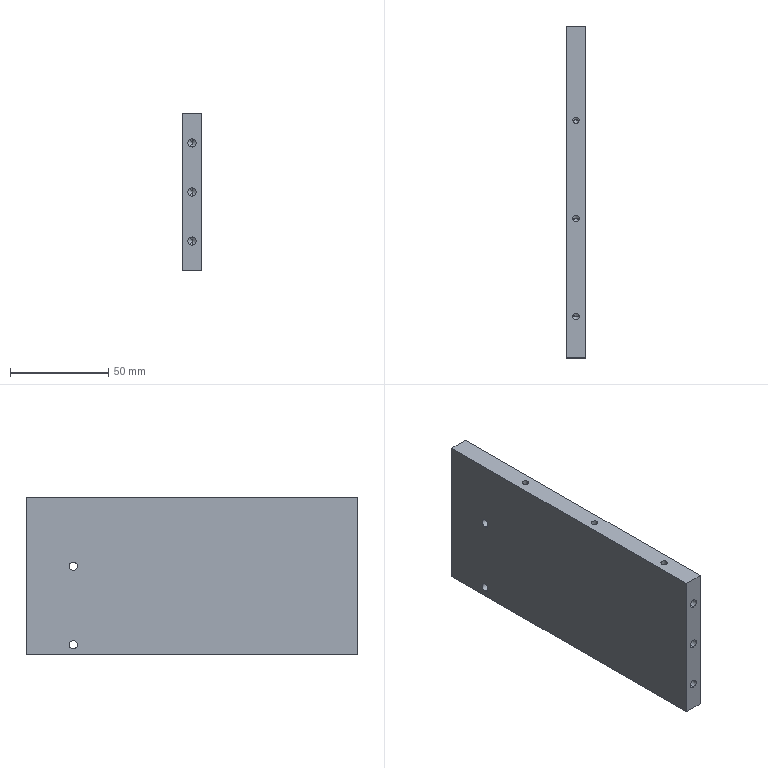Part | STEP file | 2020 Base support plate B | 1 solid | 52 faces | box 10 x 169 x 80 mm | volume 131754 mm3 | cylinder 24 | cone 18 | plane 10 | commonest cylinder face diameters 3.3 x12 4.2 x10 3 x2